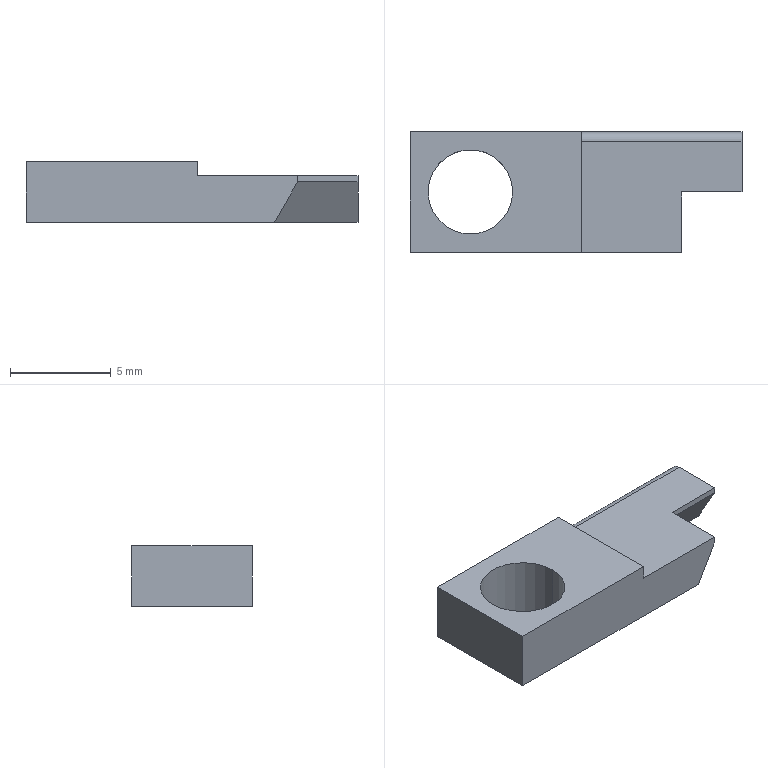Part | SolidWorks | features BaseBody 1 | 1 solid | 15 faces | box 16.5 x 6 x 3 mm | volume 192.89 mm3 | plane 12 | cylinder 3 | commonest cylinder face diameters 4.2 x2 1 x1
STEP:
#1=CARTESIAN_POINT('',(8.5,0.,2.3));
#2=VERTEX_POINT('',#1);
#3=CARTESIAN_POINT('',(8.5,0.,3.));
#4=VERTEX_POINT('',#3);
#5=CARTESIAN_POINT('',(8.5,0.,3.));
#6=DIRECTION('',(0.,0.,1.));
#7=VECTOR('',#6,1000.);
#8=LINE('',#5,#7);
#9=EDGE_CURVE('',#2,#4,#8,.T.);
#10=ORIENTED_EDGE('',*,*,#9,.F.);
#11=CARTESIAN_POINT('',(8.5,5.5,2.3));
#12=VERTEX_POINT('',#11);
#13=CARTESIAN_POINT('',(8.5,0.,2.3));
#14=DIRECTION('',(0.,1.,0.));
#15=VECTOR('',#14,1000.);
#16=LINE('',#13,#15);
#17=EDGE_CURVE('',#2,#12,#16,.T.);
#18=ORIENTED_EDGE('',*,*,#17,.T.);
#19=CARTESIAN_POINT('',(8.5,6.,1.8));
#20=VERTEX_POINT('',#19);
#21=CARTESIAN_POINT('',(8.5,5.5,1.8));
#22=DIRECTION('',(1.,0.,0.));
#23=DIRECTION('',(0.,0.,-1.));
#24=AXIS2_PLACEMENT_3D('',#21,#22,#23);
#25=CIRCLE('',#24,0.5);
#26=EDGE_CURVE('',#20,#12,#25,.T.);
#27=ORIENTED_EDGE('',*,*,#26,.F.);
#28=CARTESIAN_POINT('',(8.5,6.,3.));
#29=VERTEX_POINT('',#28);
#30=CARTESIAN_POINT('',(8.5,6.,3.));
#31=DIRECTION('',(0.,0.,-1.));
#32=VECTOR('',#31,1000.);
#33=LINE('',#30,#32);
#34=EDGE_CURVE('',#29,#20,#33,.T.);
#35=ORIENTED_EDGE('',*,*,#34,.F.);
#36=CARTESIAN_POINT('',(8.5,0.,3.));
#37=DIRECTION('',(0.,1.,0.));
#38=VECTOR('',#37,1000.);
#39=LINE('',#36,#38);
#40=EDGE_CURVE('',#4,#29,#39,.T.);
#41=ORIENTED_EDGE('',*,*,#40,.F.);
#42=EDGE_LOOP('',(#10,#18,#27,#35,#41));
#43=FACE_OUTER_BOUND('',#42,.T.);
#44=CARTESIAN_POINT('',(8.5,0.,3.));
#45=DIRECTION('',(-1.,0.,0.));
#46=DIRECTION('',(0.,0.,1.));
#47=AXIS2_PLACEMENT_3D('',#44,#45,#46);
#48=PLANE('',#47);
#49=ADVANCED_FACE('',(#43),#48,.F.);
#50=CARTESIAN_POINT('',(13.5,3.,2.3));
#51=VERTEX_POINT('',#50);
#52=CARTESIAN_POINT('',(13.5,0.,2.3));
#53=VERTEX_POINT('',#52);
#54=CARTESIAN_POINT('',(13.5,0.,2.3));
#55=DIRECTION('',(0.,-1.,0.));
#56=VECTOR('',#55,1000.);
#57=LINE('',#54,#56);
#58=EDGE_CURVE('',#51,#53,#57,.T.);
#59=ORIENTED_EDGE('',*,*,#58,.T.);
#60=CARTESIAN_POINT('',(13.5,0.,2.));
#61=VERTEX_POINT('',#60);
#62=CARTESIAN_POINT('',(13.5,0.,0.));
#63=DIRECTION('',(0.,0.,1.));
#64=VECTOR('',#63,1000.);
#65=LINE('',#62,#64);
#66=EDGE_CURVE('',#61,#53,#65,.T.);
#67=ORIENTED_EDGE('',*,*,#66,.F.);
#68=CARTESIAN_POINT('',(13.5,3.,2.));
#69=VERTEX_POINT('',#68);
#70=CARTESIAN_POINT('',(13.5,1.5,2.));
#71=DIRECTION('',(0.,-1.,0.));
#72=VECTOR('',#71,1000.);
#73=LINE('',#70,#72);
#74=EDGE_CURVE('',#69,#61,#73,.T.);
#75=ORIENTED_EDGE('',*,*,#74,.F.);
#76=CARTESIAN_POINT('',(13.5,3.,0.));
#77=DIRECTION('',(0.,0.,1.));
#78=VECTOR('',#77,1000.);
#79=LINE('',#76,#78);
#80=EDGE_CURVE('',#69,#51,#79,.T.);
#81=ORIENTED_EDGE('',*,*,#80,.T.);
#82=EDGE_LOOP('',(#59,#67,#75,#81));
#83=FACE_OUTER_BOUND('',#82,.T.);
#84=CARTESIAN_POINT('',(13.5,0.,0.));
#85=DIRECTION('',(-1.,0.,0.));
#86=DIRECTION('',(0.,0.,1.));
#87=AXIS2_PLACEMENT_3D('',#84,#85,#86);
#88=PLANE('',#87);
#89=ADVANCED_FACE('',(#83),#88,.F.);
#90=CARTESIAN_POINT('',(16.5,3.,2.3));
#91=VERTEX_POINT('',#90);
#92=CARTESIAN_POINT('',(8.5,3.,2.3));
#93=DIRECTION('',(-1.,0.,0.));
#94=VECTOR('',#93,1000.);
#95=LINE('',#92,#94);
#96=EDGE_CURVE('',#91,#51,#95,.T.);
#97=ORIENTED_EDGE('',*,*,#96,.T.);
#98=ORIENTED_EDGE('',*,*,#80,.F.);
#99=CARTESIAN_POINT('',(16.5,3.,2.));
#100=VERTEX_POINT('',#99);
#101=CARTESIAN_POINT('',(15.,3.,2.));
#102=DIRECTION('',(-1.,0.,0.));
#103=VECTOR('',#102,1000.);
#104=LINE('',#101,#103);
#105=EDGE_CURVE('',#100,#69,#104,.T.);
#106=ORIENTED_EDGE('',*,*,#105,.F.);
#107=CARTESIAN_POINT('',(16.5,3.,0.));
#108=DIRECTION('',(0.,0.,-1.));
#109=VECTOR('',#108,1000.);
#110=LINE('',#107,#109);
#111=EDGE_CURVE('',#91,#100,#110,.T.);
#112=ORIENTED_EDGE('',*,*,#111,.F.);
#113=EDGE_LOOP('',(#97,#98,#106,#112));
#114=FACE_OUTER_BOUND('',#113,.T.);
#115=CARTESIAN_POINT('',(13.5,3.,0.));
#116=DIRECTION('',(0.,1.,0.));
#117=DIRECTION('',(1.,0.,0.));
#118=AXIS2_PLACEMENT_3D('',#115,#116,#117);
#119=PLANE('',#118);
#120=ADVANCED_FACE('',(#114),#119,.F.);
#121=CARTESIAN_POINT('',(0.,0.,2.3));
#122=DIRECTION('',(-1.,0.,0.));
#123=VECTOR('',#122,1000.);
#124=LINE('',#121,#123);
#125=EDGE_CURVE('',#53,#2,#124,.T.);
#126=ORIENTED_EDGE('',*,*,#125,.F.);
#127=ORIENTED_EDGE('',*,*,#58,.F.);
#128=ORIENTED_EDGE('',*,*,#96,.F.);
#129=CARTESIAN_POINT('',(16.5,5.5,2.3));
#130=VERTEX_POINT('',#129);
#131=CARTESIAN_POINT('',(16.5,0.,2.3));
#132=DIRECTION('',(0.,-1.,0.));
#133=VECTOR('',#132,1000.);
#134=LINE('',#131,#133);
#135=EDGE_CURVE('',#130,#91,#134,.T.);
#136=ORIENTED_EDGE('',*,*,#135,.F.);
#137=CARTESIAN_POINT('',(-21.509,5.5,2.3));
#138=DIRECTION('',(1.,0.,0.));
#139=VECTOR('',#138,1000.);
#140=LINE('',#137,#139);
#141=EDGE_CURVE('',#12,#130,#140,.T.);
#142=ORIENTED_EDGE('',*,*,#141,.F.);
#143=ORIENTED_EDGE('',*,*,#17,.F.);
#144=EDGE_LOOP('',(#126,#127,#128,#136,#142,#143));
#145=FACE_OUTER_BOUND('',#144,.T.);
#146=CARTESIAN_POINT('',(8.5,0.,2.3));
#147=DIRECTION('',(0.,0.,-1.));
#148=DIRECTION('',(0.,-1.,0.));
#149=AXIS2_PLACEMENT_3D('',#146,#147,#148);
#150=PLANE('',#149);
#151=ADVANCED_FACE('',(#145),#150,.F.);
#152=ORIENTED_EDGE('',*,*,#141,.T.);
#153=CARTESIAN_POINT('',(16.5,6.,1.8));
#154=VERTEX_POINT('',#153);
#155=CARTESIAN_POINT('',(16.5,5.5,1.8));
#156=DIRECTION('',(1.,0.,0.));
#157=DIRECTION('',(0.,0.,-1.));
#158=AXIS2_PLACEMENT_3D('',#155,#156,#157);
#159=CIRCLE('',#158,0.5);
#160=EDGE_CURVE('',#154,#130,#159,.T.);
#161=ORIENTED_EDGE('',*,*,#160,.F.);
#162=CARTESIAN_POINT('',(16.5,6.,1.8));
#163=DIRECTION('',(1.,0.,0.));
#164=VECTOR('',#163,1000.);
#165=LINE('',#162,#164);
#166=EDGE_CURVE('',#20,#154,#165,.T.);
#167=ORIENTED_EDGE('',*,*,#166,.F.);
#168=ORIENTED_EDGE('',*,*,#26,.T.);
#169=EDGE_LOOP('',(#152,#161,#167,#168));
#170=FACE_OUTER_BOUND('',#169,.T.);
#171=CARTESIAN_POINT('',(-21.509,5.5,1.8));
#172=DIRECTION('',(1.,0.,0.));
#173=DIRECTION('',(0.,0.,-1.));
#174=AXIS2_PLACEMENT_3D('',#171,#172,#173);
#175=CYLINDRICAL_SURFACE('',#174,0.5);
#176=ADVANCED_FACE('',(#170),#175,.T.);
#177=CARTESIAN_POINT('',(0.9,3.,3.));
#178=VERTEX_POINT('',#177);
#179=CARTESIAN_POINT('',(5.1,3.,3.));
#180=VERTEX_POINT('',#179);
#181=CARTESIAN_POINT('',(3.,3.,3.));
#182=DIRECTION('',(0.,0.,-1.));
#183=DIRECTION('',(-1.,0.,0.));
#184=AXIS2_PLACEMENT_3D('',#181,#182,#183);
#185=CIRCLE('',#184,2.1);
#186=EDGE_CURVE('',#178,#180,#185,.T.);
#187=ORIENTED_EDGE('',*,*,#186,.T.);
#188=CARTESIAN_POINT('',(3.,3.,3.));
#189=DIRECTION('',(0.,0.,-1.));
#190=DIRECTION('',(-1.,0.,0.));
#191=AXIS2_PLACEMENT_3D('',#188,#189,#190);
#192=CIRCLE('',#191,2.1);
#193=EDGE_CURVE('',#180,#178,#192,.T.);
#194=ORIENTED_EDGE('',*,*,#193,.T.);
#195=EDGE_LOOP('',(#187,#194));
#196=FACE_BOUND('',#195,.T.);
#197=CARTESIAN_POINT('',(0.,0.,3.));
#198=VERTEX_POINT('',#197);
#199=CARTESIAN_POINT('',(0.,0.,3.));
#200=DIRECTION('',(-1.,0.,0.));
#201=VECTOR('',#200,1000.);
#202=LINE('',#199,#201);
#203=EDGE_CURVE('',#4,#198,#202,.T.);
#204=ORIENTED_EDGE('',*,*,#203,.F.);
#205=ORIENTED_EDGE('',*,*,#40,.T.);
#206=CARTESIAN_POINT('',(0.,6.,3.));
#207=VERTEX_POINT('',#206);
#208=CARTESIAN_POINT('',(16.5,6.,3.));
#209=DIRECTION('',(1.,0.,0.));
#210=VECTOR('',#209,1000.);
#211=LINE('',#208,#210);
#212=EDGE_CURVE('',#207,#29,#211,.T.);
#213=ORIENTED_EDGE('',*,*,#212,.F.);
#214=CARTESIAN_POINT('',(0.,6.,3.));
#215=DIRECTION('',(0.,1.,0.));
#216=VECTOR('',#215,1000.);
#217=LINE('',#214,#216);
#218=EDGE_CURVE('',#198,#207,#217,.T.);
#219=ORIENTED_EDGE('',*,*,#218,.F.);
#220=EDGE_LOOP('',(#204,#205,#213,#219));
#221=FACE_OUTER_BOUND('',#220,.T.);
#222=CARTESIAN_POINT('',(0.,0.,3.));
#223=DIRECTION('',(0.,0.,1.));
#224=DIRECTION('',(1.,0.,0.));
#225=AXIS2_PLACEMENT_3D('',#222,#223,#224);
#226=PLANE('',#225);
#227=ADVANCED_FACE('',(#196,#221),#226,.T.);
#228=CARTESIAN_POINT('',(0.,0.,0.));
#229=VERTEX_POINT('',#228);
#230=CARTESIAN_POINT('',(0.,0.,0.));
#231=DIRECTION('',(0.,0.,1.));
#232=VECTOR('',#231,1000.);
#233=LINE('',#230,#232);
#234=EDGE_CURVE('',#229,#198,#233,.T.);
#235=ORIENTED_EDGE('',*,*,#234,.F.);
#236=CARTESIAN_POINT('',(12.345,0.,0.));
#237=VERTEX_POINT('',#236);
#238=CARTESIAN_POINT('',(0.,0.,0.));
#239=DIRECTION('',(1.,0.,0.));
#240=VECTOR('',#239,1000.);
#241=LINE('',#238,#240);
#242=EDGE_CURVE('',#229,#237,#241,.T.);
#243=ORIENTED_EDGE('',*,*,#242,.T.);
#244=CARTESIAN_POINT('',(12.923,0.,1.));
#245=DIRECTION('',(-0.5,0.,-0.866));
#246=VECTOR('',#245,1000.);
#247=LINE('',#244,#246);
#248=EDGE_CURVE('',#61,#237,#247,.T.);
#249=ORIENTED_EDGE('',*,*,#248,.F.);
#250=ORIENTED_EDGE('',*,*,#66,.T.);
#251=ORIENTED_EDGE('',*,*,#125,.T.);
#252=ORIENTED_EDGE('',*,*,#9,.T.);
#253=ORIENTED_EDGE('',*,*,#203,.T.);
#254=EDGE_LOOP('',(#235,#243,#249,#250,#251,#252,#253));
#255=FACE_OUTER_BOUND('',#254,.T.);
#256=CARTESIAN_POINT('',(0.,0.,0.));
#257=DIRECTION('',(0.,-1.,0.));
#258=DIRECTION('',(0.,0.,-1.));
#259=AXIS2_PLACEMENT_3D('',#256,#257,#258);
#260=PLANE('',#259);
#261=ADVANCED_FACE('',(#255),#260,.T.);
#262=ORIENTED_EDGE('',*,*,#74,.T.);
#263=ORIENTED_EDGE('',*,*,#248,.T.);
#264=CARTESIAN_POINT('',(12.345,4.155,0.));
#265=VERTEX_POINT('',#264);
#266=CARTESIAN_POINT('',(12.345,0.,0.));
#267=DIRECTION('',(0.,1.,0.));
#268=VECTOR('',#267,1000.);
#269=LINE('',#266,#268);
#270=EDGE_CURVE('',#237,#265,#269,.T.);
#271=ORIENTED_EDGE('',*,*,#270,.T.);
#272=CARTESIAN_POINT('',(13.5,3.,2.));
#273=DIRECTION('',(-0.4472,0.4472,-0.7746));
#274=VECTOR('',#273,1000.);
#275=LINE('',#272,#274);
#276=EDGE_CURVE('',#69,#265,#275,.T.);
#277=ORIENTED_EDGE('',*,*,#276,.F.);
#278=EDGE_LOOP('',(#262,#263,#271,#277));
#279=FACE_OUTER_BOUND('',#278,.T.);
#280=CARTESIAN_POINT('',(12.923,1.5,1.));
#281=DIRECTION('',(0.866,0.,-0.5));
#282=DIRECTION('',(0.,-1.,0.));
#283=AXIS2_PLACEMENT_3D('',#280,#281,#282);
#284=PLANE('',#283);
#285=ADVANCED_FACE('',(#279),#284,.T.);
#286=CARTESIAN_POINT('',(16.5,4.155,0.));
#287=VERTEX_POINT('',#286);
#288=CARTESIAN_POINT('',(0.,4.155,0.));
#289=DIRECTION('',(1.,0.,0.));
#290=VECTOR('',#289,1000.);
#291=LINE('',#288,#290);
#292=EDGE_CURVE('',#265,#287,#291,.T.);
#293=ORIENTED_EDGE('',*,*,#292,.T.);
#294=CARTESIAN_POINT('',(16.5,3.,2.));
#295=DIRECTION('',(0.,0.5,-0.866));
#296=VECTOR('',#295,1000.);
#297=LINE('',#294,#296);
#298=EDGE_CURVE('',#100,#287,#297,.T.);
#299=ORIENTED_EDGE('',*,*,#298,.F.);
#300=ORIENTED_EDGE('',*,*,#105,.T.);
#301=ORIENTED_EDGE('',*,*,#276,.T.);
#302=EDGE_LOOP('',(#293,#299,#300,#301));
#303=FACE_OUTER_BOUND('',#302,.T.);
#304=CARTESIAN_POINT('',(15.,3.577,1.));
#305=DIRECTION('',(0.,-0.866,-0.5));
#306=DIRECTION('',(0.,0.5,-0.866));
#307=AXIS2_PLACEMENT_3D('',#304,#305,#306);
#308=PLANE('',#307);
#309=ADVANCED_FACE('',(#303),#308,.T.);
#310=CARTESIAN_POINT('',(16.5,6.,0.));
#311=VERTEX_POINT('',#310);
#312=CARTESIAN_POINT('',(16.5,6.,0.));
#313=DIRECTION('',(0.,0.,-1.));
#314=VECTOR('',#313,1000.);
#315=LINE('',#312,#314);
#316=EDGE_CURVE('',#154,#311,#315,.T.);
#317=ORIENTED_EDGE('',*,*,#316,.F.);
#318=ORIENTED_EDGE('',*,*,#160,.T.);
#319=ORIENTED_EDGE('',*,*,#135,.T.);
#320=ORIENTED_EDGE('',*,*,#111,.T.);
#321=ORIENTED_EDGE('',*,*,#298,.T.);
#322=CARTESIAN_POINT('',(16.5,0.,0.));
#323=DIRECTION('',(0.,1.,0.));
#324=VECTOR('',#323,1000.);
#325=LINE('',#322,#324);
#326=EDGE_CURVE('',#287,#311,#325,.T.);
#327=ORIENTED_EDGE('',*,*,#326,.T.);
#328=EDGE_LOOP('',(#317,#318,#319,#320,#321,#327));
#329=FACE_OUTER_BOUND('',#328,.T.);
#330=CARTESIAN_POINT('',(16.5,0.,0.));
#331=DIRECTION('',(1.,0.,0.));
#332=DIRECTION('',(0.,1.,0.));
#333=AXIS2_PLACEMENT_3D('',#330,#331,#332);
#334=PLANE('',#333);
#335=ADVANCED_FACE('',(#329),#334,.T.);
#336=ORIENTED_EDGE('',*,*,#34,.T.);
#337=ORIENTED_EDGE('',*,*,#166,.T.);
#338=ORIENTED_EDGE('',*,*,#316,.T.);
#339=CARTESIAN_POINT('',(0.,6.,0.));
#340=VERTEX_POINT('',#339);
#341=CARTESIAN_POINT('',(0.,6.,0.));
#342=DIRECTION('',(-1.,0.,0.));
#343=VECTOR('',#342,1000.);
#344=LINE('',#341,#343);
#345=EDGE_CURVE('',#311,#340,#344,.T.);
#346=ORIENTED_EDGE('',*,*,#345,.T.);
#347=CARTESIAN_POINT('',(0.,6.,0.));
#348=DIRECTION('',(0.,0.,-1.));
#349=VECTOR('',#348,1000.);
#350=LINE('',#347,#349);
#351=EDGE_CURVE('',#207,#340,#350,.T.);
#352=ORIENTED_EDGE('',*,*,#351,.F.);
#353=ORIENTED_EDGE('',*,*,#212,.T.);
#354=EDGE_LOOP('',(#336,#337,#338,#346,#352,#353));
#355=FACE_OUTER_BOUND('',#354,.T.);
#356=CARTESIAN_POINT('',(16.5,6.,0.));
#357=DIRECTION('',(0.,1.,0.));
#358=DIRECTION('',(1.,0.,0.));
#359=AXIS2_PLACEMENT_3D('',#356,#357,#358);
#360=PLANE('',#359);
#361=ADVANCED_FACE('',(#355),#360,.T.);
#362=ORIENTED_EDGE('',*,*,#351,.T.);
#363=CARTESIAN_POINT('',(0.,0.,0.));
#364=DIRECTION('',(0.,-1.,0.));
#365=VECTOR('',#364,1000.);
#366=LINE('',#363,#365);
#367=EDGE_CURVE('',#340,#229,#366,.T.);
#368=ORIENTED_EDGE('',*,*,#367,.T.);
#369=ORIENTED_EDGE('',*,*,#234,.T.);
#370=ORIENTED_EDGE('',*,*,#218,.T.);
#371=EDGE_LOOP('',(#362,#368,#369,#370));
#372=FACE_OUTER_BOUND('',#371,.T.);
#373=CARTESIAN_POINT('',(0.,6.,0.));
#374=DIRECTION('',(-1.,0.,0.));
#375=DIRECTION('',(0.,0.,1.));
#376=AXIS2_PLACEMENT_3D('',#373,#374,#375);
#377=PLANE('',#376);
#378=ADVANCED_FACE('',(#372),#377,.T.);
#379=CARTESIAN_POINT('',(5.1,3.,0.));
#380=VERTEX_POINT('',#379);
#381=CARTESIAN_POINT('',(5.1,3.,0.));
#382=DIRECTION('',(0.,0.,-1.));
#383=VECTOR('',#382,1000.);
#384=LINE('',#381,#383);
#385=EDGE_CURVE('',#180,#380,#384,.T.);
#386=ORIENTED_EDGE('',*,*,#385,.F.);
#387=ORIENTED_EDGE('',*,*,#186,.F.);
#388=CARTESIAN_POINT('',(0.9,3.,0.));
#389=VERTEX_POINT('',#388);
#390=CARTESIAN_POINT('',(0.9,3.,0.));
#391=DIRECTION('',(0.,0.,-1.));
#392=VECTOR('',#391,1000.);
#393=LINE('',#390,#392);
#394=EDGE_CURVE('',#178,#389,#393,.T.);
#395=ORIENTED_EDGE('',*,*,#394,.T.);
#396=CARTESIAN_POINT('',(3.,3.,0.));
#397=DIRECTION('',(0.,0.,-1.));
#398=DIRECTION('',(-1.,0.,0.));
#399=AXIS2_PLACEMENT_3D('',#396,#397,#398);
#400=CIRCLE('',#399,2.1);
#401=EDGE_CURVE('',#389,#380,#400,.T.);
#402=ORIENTED_EDGE('',*,*,#401,.T.);
#403=EDGE_LOOP('',(#386,#387,#395,#402));
#404=FACE_OUTER_BOUND('',#403,.T.);
#405=CARTESIAN_POINT('',(3.,3.,0.));
#406=DIRECTION('',(0.,0.,-1.));
#407=DIRECTION('',(-1.,0.,0.));
#408=AXIS2_PLACEMENT_3D('',#405,#406,#407);
#409=CYLINDRICAL_SURFACE('',#408,2.1);
#410=ADVANCED_FACE('',(#404),#409,.F.);
#411=ORIENTED_EDGE('',*,*,#401,.F.);
#412=CARTESIAN_POINT('',(3.,3.,0.));
#413=DIRECTION('',(0.,0.,-1.));
#414=DIRECTION('',(-1.,0.,0.));
#415=AXIS2_PLACEMENT_3D('',#412,#413,#414);
#416=CIRCLE('',#415,2.1);
#417=EDGE_CURVE('',#380,#389,#416,.T.);
#418=ORIENTED_EDGE('',*,*,#417,.F.);
#419=EDGE_LOOP('',(#411,#418));
#420=FACE_BOUND('',#419,.T.);
#421=ORIENTED_EDGE('',*,*,#345,.F.);
#422=ORIENTED_EDGE('',*,*,#326,.F.);
#423=ORIENTED_EDGE('',*,*,#292,.F.);
#424=ORIENTED_EDGE('',*,*,#270,.F.);
#425=ORIENTED_EDGE('',*,*,#242,.F.);
#426=ORIENTED_EDGE('',*,*,#367,.F.);
#427=EDGE_LOOP('',(#421,#422,#423,#424,#425,#426));
#428=FACE_OUTER_BOUND('',#427,.T.);
#429=CARTESIAN_POINT('',(0.,0.,0.));
#430=DIRECTION('',(0.,0.,1.));
#431=DIRECTION('',(1.,0.,0.));
#432=AXIS2_PLACEMENT_3D('',#429,#430,#431);
#433=PLANE('',#432);
#434=ADVANCED_FACE('',(#420,#428),#433,.F.);
#435=ORIENTED_EDGE('',*,*,#193,.F.);
#436=ORIENTED_EDGE('',*,*,#385,.T.);
#437=ORIENTED_EDGE('',*,*,#417,.T.);
#438=ORIENTED_EDGE('',*,*,#394,.F.);
#439=EDGE_LOOP('',(#435,#436,#437,#438));
#440=FACE_OUTER_BOUND('',#439,.T.);
#441=CARTESIAN_POINT('',(3.,3.,0.));
#442=DIRECTION('',(0.,0.,-1.));
#443=DIRECTION('',(-1.,0.,0.));
#444=AXIS2_PLACEMENT_3D('',#441,#442,#443);
#445=CYLINDRICAL_SURFACE('',#444,2.1);
#446=ADVANCED_FACE('',(#440),#445,.F.);
#447=CLOSED_SHELL('',(#49,#89,#120,#151,#176,#227,#261,#285,#309,#335,#361,#378,#410,#434,#446));
#448=MANIFOLD_SOLID_BREP('',#447);
#449=CARTESIAN_POINT('',(0.,0.,0.));
#450=DIRECTION('',(0.,0.,1.));
#451=DIRECTION('',(1.,0.,0.));
#452=AXIS2_PLACEMENT_3D('',#449,#450,#451);
#453=(LENGTH_UNIT()NAMED_UNIT(*)SI_UNIT(.MILLI.,.METRE.));
#454=UNCERTAINTY_MEASURE_WITH_UNIT(LENGTH_MEASURE(0.00001),#453,'','');
#455=(NAMED_UNIT(*)PLANE_ANGLE_UNIT()SI_UNIT($,.RADIAN.));
#456=(NAMED_UNIT(*)SI_UNIT($,.STERADIAN.)SOLID_ANGLE_UNIT());
#457=(GEOMETRIC_REPRESENTATION_CONTEXT(3)GLOBAL_UNCERTAINTY_ASSIGNED_CONTEXT((#454))GLOBAL_UNIT_ASSIGNED_CONTEXT((#453,#455,#456))REPRESENTATION_CONTEXT('',''));
#458=ADVANCED_BREP_SHAPE_REPRESENTATION('',(#448,#452),#457);